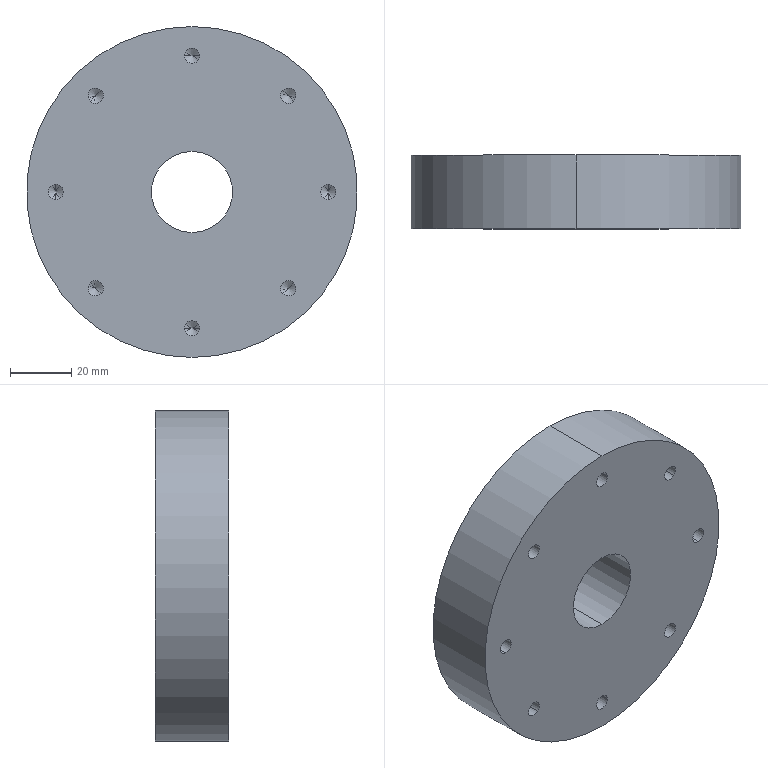Part | STEP file | 1 solid | 38 faces | box 108 x 24 x 108 mm | volume 204189 mm3 | cylinder 20 | cone 16 | plane 2 | commonest cylinder face diameters 5 x16 26.5 x2 108 x2